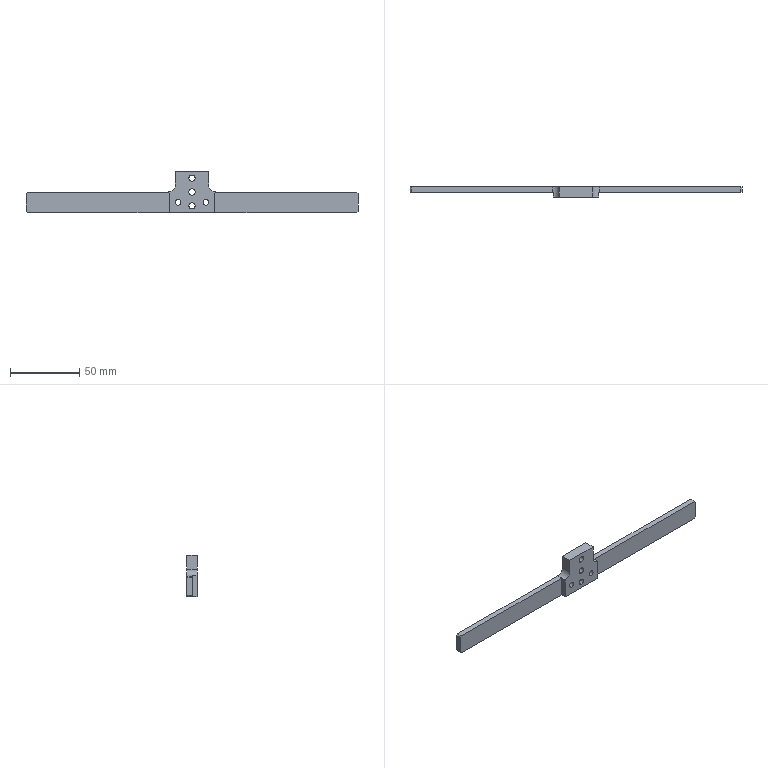Part | SolidWorks | features ICE 6, LPattern 2, Chamfer 1, Extrusion 1, Fillet 1, HoleWzd 1 | 1 solid | 30 faces | box 240 x 7.5 x 30 mm | volume 18359 mm3 | plane 18 | cylinder 12 | commonest cylinder face diameters 4.5 x6 4 x4 10 x2
STEP:
#1=CARTESIAN_POINT('',(-80.,-5.5,-9.5));
#2=VERTEX_POINT('',#1);
#3=CARTESIAN_POINT('',(-80.,-5.5,-5.5));
#4=VERTEX_POINT('',#3);
#5=CARTESIAN_POINT('',(-80.,-5.5,-7.5));
#6=DIRECTION('',(0.,1.,0.));
#7=DIRECTION('',(0.,0.,1.));
#8=AXIS2_PLACEMENT_3D('',#5,#6,#7);
#9=CIRCLE('',#8,2.);
#10=EDGE_CURVE('',#2,#4,#9,.T.);
#11=ORIENTED_EDGE('',*,*,#10,.F.);
#12=CARTESIAN_POINT('',(-80.,2.,-9.5));
#13=VERTEX_POINT('',#12);
#14=CARTESIAN_POINT('',(-80.,2.,-9.5));
#15=DIRECTION('',(0.,1.,0.));
#16=VECTOR('',#15,1000.);
#17=LINE('',#14,#16);
#18=EDGE_CURVE('',#2,#13,#17,.T.);
#19=ORIENTED_EDGE('',*,*,#18,.T.);
#20=CARTESIAN_POINT('',(-80.,2.,-5.5));
#21=VERTEX_POINT('',#20);
#22=CARTESIAN_POINT('',(-80.,2.,-7.5));
#23=DIRECTION('',(0.,1.,0.));
#24=DIRECTION('',(0.,0.,1.));
#25=AXIS2_PLACEMENT_3D('',#22,#23,#24);
#26=CIRCLE('',#25,2.);
#27=EDGE_CURVE('',#13,#21,#26,.T.);
#28=ORIENTED_EDGE('',*,*,#27,.T.);
#29=CARTESIAN_POINT('',(-80.,2.,-5.5));
#30=DIRECTION('',(0.,1.,0.));
#31=VECTOR('',#30,1000.);
#32=LINE('',#29,#31);
#33=EDGE_CURVE('',#4,#21,#32,.T.);
#34=ORIENTED_EDGE('',*,*,#33,.F.);
#35=EDGE_LOOP('',(#11,#19,#28,#34));
#36=FACE_OUTER_BOUND('',#35,.T.);
#37=CARTESIAN_POINT('',(-80.,2.,-7.5));
#38=DIRECTION('',(0.,1.,0.));
#39=DIRECTION('',(0.,0.,1.));
#40=AXIS2_PLACEMENT_3D('',#37,#38,#39);
#41=CYLINDRICAL_SURFACE('',#40,2.);
#42=ADVANCED_FACE('',(#36),#41,.F.);
#43=CARTESIAN_POINT('',(-60.,-5.5,-9.5));
#44=VERTEX_POINT('',#43);
#45=CARTESIAN_POINT('',(-60.,-5.5,-5.5));
#46=VERTEX_POINT('',#45);
#47=CARTESIAN_POINT('',(-60.,-5.5,-7.5));
#48=DIRECTION('',(0.,1.,0.));
#49=DIRECTION('',(0.,0.,1.));
#50=AXIS2_PLACEMENT_3D('',#47,#48,#49);
#51=CIRCLE('',#50,2.);
#52=EDGE_CURVE('',#44,#46,#51,.T.);
#53=ORIENTED_EDGE('',*,*,#52,.F.);
#54=CARTESIAN_POINT('',(-60.,2.,-9.5));
#55=VERTEX_POINT('',#54);
#56=CARTESIAN_POINT('',(-60.,2.,-9.5));
#57=DIRECTION('',(0.,1.,0.));
#58=VECTOR('',#57,1000.);
#59=LINE('',#56,#58);
#60=EDGE_CURVE('',#44,#55,#59,.T.);
#61=ORIENTED_EDGE('',*,*,#60,.T.);
#62=CARTESIAN_POINT('',(-60.,2.,-5.5));
#63=VERTEX_POINT('',#62);
#64=CARTESIAN_POINT('',(-60.,2.,-7.5));
#65=DIRECTION('',(0.,1.,0.));
#66=DIRECTION('',(0.,0.,1.));
#67=AXIS2_PLACEMENT_3D('',#64,#65,#66);
#68=CIRCLE('',#67,2.);
#69=EDGE_CURVE('',#55,#63,#68,.T.);
#70=ORIENTED_EDGE('',*,*,#69,.T.);
#71=CARTESIAN_POINT('',(-60.,2.,-5.5));
#72=DIRECTION('',(0.,1.,0.));
#73=VECTOR('',#72,1000.);
#74=LINE('',#71,#73);
#75=EDGE_CURVE('',#46,#63,#74,.T.);
#76=ORIENTED_EDGE('',*,*,#75,.F.);
#77=EDGE_LOOP('',(#53,#61,#70,#76));
#78=FACE_OUTER_BOUND('',#77,.T.);
#79=CARTESIAN_POINT('',(-60.,2.,-7.5));
#80=DIRECTION('',(0.,1.,0.));
#81=DIRECTION('',(0.,0.,1.));
#82=AXIS2_PLACEMENT_3D('',#79,#80,#81);
#83=CYLINDRICAL_SURFACE('',#82,2.);
#84=ADVANCED_FACE('',(#78),#83,.F.);
#85=CARTESIAN_POINT('',(-70.,-5.5,-7.75));
#86=VERTEX_POINT('',#85);
#87=CARTESIAN_POINT('',(-70.,-5.5,-12.25));
#88=VERTEX_POINT('',#87);
#89=CARTESIAN_POINT('',(-70.,-5.5,-10.));
#90=DIRECTION('',(0.,-1.,0.));
#91=DIRECTION('',(0.,0.,-1.));
#92=AXIS2_PLACEMENT_3D('',#89,#90,#91);
#93=CIRCLE('',#92,2.25);
#94=EDGE_CURVE('',#86,#88,#93,.T.);
#95=ORIENTED_EDGE('',*,*,#94,.T.);
#96=CARTESIAN_POINT('',(-70.,2.,-12.25));
#97=VERTEX_POINT('',#96);
#98=CARTESIAN_POINT('',(-70.,-5.5,-12.25));
#99=DIRECTION('',(0.,1.,0.));
#100=VECTOR('',#99,1000.);
#101=LINE('',#98,#100);
#102=EDGE_CURVE('',#88,#97,#101,.T.);
#103=ORIENTED_EDGE('',*,*,#102,.T.);
#104=CARTESIAN_POINT('',(-70.,2.,-7.75));
#105=VERTEX_POINT('',#104);
#106=CARTESIAN_POINT('',(-70.,2.,-10.));
#107=DIRECTION('',(0.,1.,0.));
#108=DIRECTION('',(0.,0.,1.));
#109=AXIS2_PLACEMENT_3D('',#106,#107,#108);
#110=CIRCLE('',#109,2.25);
#111=EDGE_CURVE('',#97,#105,#110,.T.);
#112=ORIENTED_EDGE('',*,*,#111,.T.);
#113=CARTESIAN_POINT('',(-70.,-5.5,-7.75));
#114=DIRECTION('',(0.,1.,0.));
#115=VECTOR('',#114,1000.);
#116=LINE('',#113,#115);
#117=EDGE_CURVE('',#86,#105,#116,.T.);
#118=ORIENTED_EDGE('',*,*,#117,.F.);
#119=EDGE_LOOP('',(#95,#103,#112,#118));
#120=FACE_OUTER_BOUND('',#119,.T.);
#121=CARTESIAN_POINT('',(-70.,-5.5,-10.));
#122=DIRECTION('',(0.,1.,0.));
#123=DIRECTION('',(0.,0.,1.));
#124=AXIS2_PLACEMENT_3D('',#121,#122,#123);
#125=CYLINDRICAL_SURFACE('',#124,2.25);
#126=ADVANCED_FACE('',(#120),#125,.F.);
#127=CARTESIAN_POINT('',(-70.,-5.5,2.25));
#128=VERTEX_POINT('',#127);
#129=CARTESIAN_POINT('',(-70.,-5.5,-2.25));
#130=VERTEX_POINT('',#129);
#131=CARTESIAN_POINT('',(-70.,-5.5,0.));
#132=DIRECTION('',(0.,-1.,0.));
#133=DIRECTION('',(0.,0.,-1.));
#134=AXIS2_PLACEMENT_3D('',#131,#132,#133);
#135=CIRCLE('',#134,2.25);
#136=EDGE_CURVE('',#128,#130,#135,.T.);
#137=ORIENTED_EDGE('',*,*,#136,.T.);
#138=CARTESIAN_POINT('',(-70.,2.,-2.25));
#139=VERTEX_POINT('',#138);
#140=CARTESIAN_POINT('',(-70.,-5.5,-2.25));
#141=DIRECTION('',(0.,1.,0.));
#142=VECTOR('',#141,1000.);
#143=LINE('',#140,#142);
#144=EDGE_CURVE('',#130,#139,#143,.T.);
#145=ORIENTED_EDGE('',*,*,#144,.T.);
#146=CARTESIAN_POINT('',(-70.,2.,2.25));
#147=VERTEX_POINT('',#146);
#148=CARTESIAN_POINT('',(-70.,2.,0.));
#149=DIRECTION('',(0.,1.,0.));
#150=DIRECTION('',(0.,0.,1.));
#151=AXIS2_PLACEMENT_3D('',#148,#149,#150);
#152=CIRCLE('',#151,2.25);
#153=EDGE_CURVE('',#139,#147,#152,.T.);
#154=ORIENTED_EDGE('',*,*,#153,.T.);
#155=CARTESIAN_POINT('',(-70.,-5.5,2.25));
#156=DIRECTION('',(0.,1.,0.));
#157=VECTOR('',#156,1000.);
#158=LINE('',#155,#157);
#159=EDGE_CURVE('',#128,#147,#158,.T.);
#160=ORIENTED_EDGE('',*,*,#159,.F.);
#161=EDGE_LOOP('',(#137,#145,#154,#160));
#162=FACE_OUTER_BOUND('',#161,.T.);
#163=CARTESIAN_POINT('',(-70.,-5.5,0.));
#164=DIRECTION('',(0.,1.,0.));
#165=DIRECTION('',(0.,0.,1.));
#166=AXIS2_PLACEMENT_3D('',#163,#164,#165);
#167=CYLINDRICAL_SURFACE('',#166,2.25);
#168=ADVANCED_FACE('',(#162),#167,.F.);
#169=CARTESIAN_POINT('',(-70.,-5.5,12.25));
#170=VERTEX_POINT('',#169);
#171=CARTESIAN_POINT('',(-70.,-5.5,7.75));
#172=VERTEX_POINT('',#171);
#173=CARTESIAN_POINT('',(-70.,-5.5,10.));
#174=DIRECTION('',(0.,-1.,0.));
#175=DIRECTION('',(0.,0.,-1.));
#176=AXIS2_PLACEMENT_3D('',#173,#174,#175);
#177=CIRCLE('',#176,2.25);
#178=EDGE_CURVE('',#170,#172,#177,.T.);
#179=ORIENTED_EDGE('',*,*,#178,.T.);
#180=CARTESIAN_POINT('',(-70.,2.,7.75));
#181=VERTEX_POINT('',#180);
#182=CARTESIAN_POINT('',(-70.,-5.5,7.75));
#183=DIRECTION('',(0.,1.,0.));
#184=VECTOR('',#183,1000.);
#185=LINE('',#182,#184);
#186=EDGE_CURVE('',#172,#181,#185,.T.);
#187=ORIENTED_EDGE('',*,*,#186,.T.);
#188=CARTESIAN_POINT('',(-70.,2.,12.25));
#189=VERTEX_POINT('',#188);
#190=CARTESIAN_POINT('',(-70.,2.,10.));
#191=DIRECTION('',(0.,1.,0.));
#192=DIRECTION('',(0.,0.,1.));
#193=AXIS2_PLACEMENT_3D('',#190,#191,#192);
#194=CIRCLE('',#193,2.25);
#195=EDGE_CURVE('',#181,#189,#194,.T.);
#196=ORIENTED_EDGE('',*,*,#195,.T.);
#197=CARTESIAN_POINT('',(-70.,-5.5,12.25));
#198=DIRECTION('',(0.,1.,0.));
#199=VECTOR('',#198,1000.);
#200=LINE('',#197,#199);
#201=EDGE_CURVE('',#170,#189,#200,.T.);
#202=ORIENTED_EDGE('',*,*,#201,.F.);
#203=EDGE_LOOP('',(#179,#187,#196,#202));
#204=FACE_OUTER_BOUND('',#203,.T.);
#205=CARTESIAN_POINT('',(-70.,-5.5,10.));
#206=DIRECTION('',(0.,1.,0.));
#207=DIRECTION('',(0.,0.,1.));
#208=AXIS2_PLACEMENT_3D('',#205,#206,#207);
#209=CYLINDRICAL_SURFACE('',#208,2.25);
#210=ADVANCED_FACE('',(#204),#209,.F.);
#211=CARTESIAN_POINT('',(-80.,-5.5,-7.5));
#212=DIRECTION('',(0.,1.,0.));
#213=DIRECTION('',(0.,0.,1.));
#214=AXIS2_PLACEMENT_3D('',#211,#212,#213);
#215=CIRCLE('',#214,2.);
#216=EDGE_CURVE('',#4,#2,#215,.T.);
#217=ORIENTED_EDGE('',*,*,#216,.T.);
#218=ORIENTED_EDGE('',*,*,#10,.T.);
#219=EDGE_LOOP('',(#217,#218));
#220=FACE_BOUND('',#219,.T.);
#221=ORIENTED_EDGE('',*,*,#94,.F.);
#222=CARTESIAN_POINT('',(-70.,-5.5,-10.));
#223=DIRECTION('',(0.,-1.,0.));
#224=DIRECTION('',(0.,0.,-1.));
#225=AXIS2_PLACEMENT_3D('',#222,#223,#224);
#226=CIRCLE('',#225,2.25);
#227=EDGE_CURVE('',#88,#86,#226,.T.);
#228=ORIENTED_EDGE('',*,*,#227,.F.);
#229=EDGE_LOOP('',(#221,#228));
#230=FACE_BOUND('',#229,.T.);
#231=ORIENTED_EDGE('',*,*,#178,.F.);
#232=CARTESIAN_POINT('',(-70.,-5.5,10.));
#233=DIRECTION('',(0.,-1.,0.));
#234=DIRECTION('',(0.,0.,-1.));
#235=AXIS2_PLACEMENT_3D('',#232,#233,#234);
#236=CIRCLE('',#235,2.25);
#237=EDGE_CURVE('',#172,#170,#236,.T.);
#238=ORIENTED_EDGE('',*,*,#237,.F.);
#239=EDGE_LOOP('',(#231,#238));
#240=FACE_BOUND('',#239,.T.);
#241=ORIENTED_EDGE('',*,*,#136,.F.);
#242=CARTESIAN_POINT('',(-70.,-5.5,0.));
#243=DIRECTION('',(0.,-1.,0.));
#244=DIRECTION('',(0.,0.,-1.));
#245=AXIS2_PLACEMENT_3D('',#242,#243,#244);
#246=CIRCLE('',#245,2.25);
#247=EDGE_CURVE('',#130,#128,#246,.T.);
#248=ORIENTED_EDGE('',*,*,#247,.F.);
#249=EDGE_LOOP('',(#241,#248));
#250=FACE_BOUND('',#249,.T.);
#251=CARTESIAN_POINT('',(-82.,-5.5,5.));
#252=VERTEX_POINT('',#251);
#253=CARTESIAN_POINT('',(-82.,-5.5,15.));
#254=VERTEX_POINT('',#253);
#255=CARTESIAN_POINT('',(-82.,-5.5,-15.));
#256=DIRECTION('',(0.,0.,1.));
#257=VECTOR('',#256,1000.);
#258=LINE('',#255,#257);
#259=EDGE_CURVE('',#252,#254,#258,.T.);
#260=ORIENTED_EDGE('',*,*,#259,.F.);
#261=CARTESIAN_POINT('',(-86.5,-5.5,0.02506));
#262=VERTEX_POINT('',#261);
#263=CARTESIAN_POINT('',(-87.,-5.5,5.));
#264=DIRECTION('',(0.,-1.,0.));
#265=DIRECTION('',(0.,0.,-1.));
#266=AXIS2_PLACEMENT_3D('',#263,#264,#265);
#267=CIRCLE('',#266,5.);
#268=EDGE_CURVE('',#262,#252,#267,.T.);
#269=ORIENTED_EDGE('',*,*,#268,.F.);
#270=CARTESIAN_POINT('',(-86.5,-5.5,-15.));
#271=VERTEX_POINT('',#270);
#272=CARTESIAN_POINT('',(-86.5,-5.5,-15.));
#273=DIRECTION('',(0.,0.,-1.));
#274=VECTOR('',#273,1000.);
#275=LINE('',#272,#274);
#276=EDGE_CURVE('',#262,#271,#275,.T.);
#277=ORIENTED_EDGE('',*,*,#276,.T.);
#278=CARTESIAN_POINT('',(-53.5,-5.5,-15.));
#279=VERTEX_POINT('',#278);
#280=CARTESIAN_POINT('',(-82.,-5.5,-15.));
#281=DIRECTION('',(1.,0.,0.));
#282=VECTOR('',#281,1000.);
#283=LINE('',#280,#282);
#284=EDGE_CURVE('',#271,#279,#283,.T.);
#285=ORIENTED_EDGE('',*,*,#284,.T.);
#286=CARTESIAN_POINT('',(-53.5,-5.5,0.02506));
#287=VERTEX_POINT('',#286);
#288=CARTESIAN_POINT('',(-53.5,-5.5,-15.));
#289=DIRECTION('',(0.,0.,1.));
#290=VECTOR('',#289,1000.);
#291=LINE('',#288,#290);
#292=EDGE_CURVE('',#279,#287,#291,.T.);
#293=ORIENTED_EDGE('',*,*,#292,.T.);
#294=CARTESIAN_POINT('',(-58.,-5.5,5.));
#295=VERTEX_POINT('',#294);
#296=CARTESIAN_POINT('',(-53.,-5.5,5.));
#297=DIRECTION('',(0.,-1.,0.));
#298=DIRECTION('',(0.,0.,-1.));
#299=AXIS2_PLACEMENT_3D('',#296,#297,#298);
#300=CIRCLE('',#299,5.);
#301=EDGE_CURVE('',#295,#287,#300,.T.);
#302=ORIENTED_EDGE('',*,*,#301,.F.);
#303=CARTESIAN_POINT('',(-58.,-5.5,15.));
#304=VERTEX_POINT('',#303);
#305=CARTESIAN_POINT('',(-58.,-5.5,-15.));
#306=DIRECTION('',(0.,0.,-1.));
#307=VECTOR('',#306,1000.);
#308=LINE('',#305,#307);
#309=EDGE_CURVE('',#304,#295,#308,.T.);
#310=ORIENTED_EDGE('',*,*,#309,.F.);
#311=CARTESIAN_POINT('',(-82.,-5.5,15.));
#312=DIRECTION('',(-1.,0.,0.));
#313=VECTOR('',#312,1000.);
#314=LINE('',#311,#313);
#315=EDGE_CURVE('',#304,#254,#314,.T.);
#316=ORIENTED_EDGE('',*,*,#315,.T.);
#317=EDGE_LOOP('',(#260,#269,#277,#285,#293,#302,#310,#316));
#318=FACE_OUTER_BOUND('',#317,.T.);
#319=CARTESIAN_POINT('',(-60.,-5.5,-7.5));
#320=DIRECTION('',(0.,1.,0.));
#321=DIRECTION('',(0.,0.,1.));
#322=AXIS2_PLACEMENT_3D('',#319,#320,#321);
#323=CIRCLE('',#322,2.);
#324=EDGE_CURVE('',#46,#44,#323,.T.);
#325=ORIENTED_EDGE('',*,*,#324,.T.);
#326=ORIENTED_EDGE('',*,*,#52,.T.);
#327=EDGE_LOOP('',(#325,#326));
#328=FACE_BOUND('',#327,.T.);
#329=CARTESIAN_POINT('',(-82.,-5.5,-15.));
#330=DIRECTION('',(0.,-1.,0.));
#331=DIRECTION('',(0.,0.,-1.));
#332=AXIS2_PLACEMENT_3D('',#329,#330,#331);
#333=PLANE('',#332);
#334=ADVANCED_FACE('',(#220,#230,#240,#250,#318,#328),#333,.T.);
#335=CARTESIAN_POINT('',(-189.,-2.,-15.));
#336=VERTEX_POINT('',#335);
#337=CARTESIAN_POINT('',(-86.5,-2.,-15.));
#338=VERTEX_POINT('',#337);
#339=CARTESIAN_POINT('',(-69.,-2.,-15.));
#340=DIRECTION('',(1.,0.,0.));
#341=VECTOR('',#340,1000.);
#342=LINE('',#339,#341);
#343=EDGE_CURVE('',#336,#338,#342,.T.);
#344=ORIENTED_EDGE('',*,*,#343,.T.);
#345=CARTESIAN_POINT('',(-86.5,-2.,0.02506));
#346=VERTEX_POINT('',#345);
#347=CARTESIAN_POINT('',(-86.5,-2.,-15.));
#348=DIRECTION('',(0.,0.,-1.));
#349=VECTOR('',#348,1000.);
#350=LINE('',#347,#349);
#351=EDGE_CURVE('',#346,#338,#350,.T.);
#352=ORIENTED_EDGE('',*,*,#351,.F.);
#353=CARTESIAN_POINT('',(-87.,-2.,0.));
#354=VERTEX_POINT('',#353);
#355=CARTESIAN_POINT('',(-87.,-2.,5.));
#356=DIRECTION('',(0.,1.,0.));
#357=DIRECTION('',(0.,0.,1.));
#358=AXIS2_PLACEMENT_3D('',#355,#356,#357);
#359=CIRCLE('',#358,5.);
#360=EDGE_CURVE('',#346,#354,#359,.T.);
#361=ORIENTED_EDGE('',*,*,#360,.T.);
#362=CARTESIAN_POINT('',(-189.,-2.,0.));
#363=VERTEX_POINT('',#362);
#364=CARTESIAN_POINT('',(-190.,-2.,0.));
#365=DIRECTION('',(1.,0.,0.));
#366=VECTOR('',#365,1000.);
#367=LINE('',#364,#366);
#368=EDGE_CURVE('',#363,#354,#367,.T.);
#369=ORIENTED_EDGE('',*,*,#368,.F.);
#370=CARTESIAN_POINT('',(-190.,-2.,-1.));
#371=VERTEX_POINT('',#370);
#372=CARTESIAN_POINT('',(-190.,-2.,-1.));
#373=DIRECTION('',(-0.7071,0.,-0.7071));
#374=VECTOR('',#373,1000.);
#375=LINE('',#372,#374);
#376=EDGE_CURVE('',#363,#371,#375,.T.);
#377=ORIENTED_EDGE('',*,*,#376,.T.);
#378=CARTESIAN_POINT('',(-190.,-2.,-14.));
#379=VERTEX_POINT('',#378);
#380=CARTESIAN_POINT('',(-190.,-2.,-15.));
#381=DIRECTION('',(0.,0.,1.));
#382=VECTOR('',#381,1000.);
#383=LINE('',#380,#382);
#384=EDGE_CURVE('',#379,#371,#383,.T.);
#385=ORIENTED_EDGE('',*,*,#384,.F.);
#386=CARTESIAN_POINT('',(-189.,-2.,-15.));
#387=DIRECTION('',(0.7071,0.,-0.7071));
#388=VECTOR('',#387,1000.);
#389=LINE('',#386,#388);
#390=EDGE_CURVE('',#379,#336,#389,.T.);
#391=ORIENTED_EDGE('',*,*,#390,.T.);
#392=EDGE_LOOP('',(#344,#352,#361,#369,#377,#385,#391));
#393=FACE_OUTER_BOUND('',#392,.T.);
#394=CARTESIAN_POINT('',(-53.,-2.,5.));
#395=DIRECTION('',(0.,1.,0.));
#396=DIRECTION('',(0.,0.,1.));
#397=AXIS2_PLACEMENT_3D('',#394,#395,#396);
#398=PLANE('',#397);
#399=ADVANCED_FACE('',(#393),#398,.F.);
#400=CARTESIAN_POINT('',(-53.,-2.,0.));
#401=VERTEX_POINT('',#400);
#402=CARTESIAN_POINT('',(-53.5,-2.,0.02506));
#403=VERTEX_POINT('',#402);
#404=CARTESIAN_POINT('',(-53.,-2.,5.));
#405=DIRECTION('',(0.,1.,0.));
#406=DIRECTION('',(0.,0.,1.));
#407=AXIS2_PLACEMENT_3D('',#404,#405,#406);
#408=CIRCLE('',#407,5.);
#409=EDGE_CURVE('',#401,#403,#408,.T.);
#410=ORIENTED_EDGE('',*,*,#409,.T.);
#411=CARTESIAN_POINT('',(-53.5,-2.,-15.));
#412=VERTEX_POINT('',#411);
#413=CARTESIAN_POINT('',(-53.5,-2.,-15.));
#414=DIRECTION('',(0.,0.,1.));
#415=VECTOR('',#414,1000.);
#416=LINE('',#413,#415);
#417=EDGE_CURVE('',#412,#403,#416,.T.);
#418=ORIENTED_EDGE('',*,*,#417,.F.);
#419=CARTESIAN_POINT('',(49.,-2.,-15.));
#420=VERTEX_POINT('',#419);
#421=CARTESIAN_POINT('',(-69.,-2.,-15.));
#422=DIRECTION('',(1.,0.,0.));
#423=VECTOR('',#422,1000.);
#424=LINE('',#421,#423);
#425=EDGE_CURVE('',#412,#420,#424,.T.);
#426=ORIENTED_EDGE('',*,*,#425,.T.);
#427=CARTESIAN_POINT('',(50.,-2.,-14.));
#428=VERTEX_POINT('',#427);
#429=CARTESIAN_POINT('',(50.,-2.,-14.));
#430=DIRECTION('',(0.7071,0.,0.7071));
#431=VECTOR('',#430,1000.);
#432=LINE('',#429,#431);
#433=EDGE_CURVE('',#420,#428,#432,.T.);
#434=ORIENTED_EDGE('',*,*,#433,.T.);
#435=CARTESIAN_POINT('',(50.,-2.,-1.));
#436=VERTEX_POINT('',#435);
#437=CARTESIAN_POINT('',(50.,-2.,5.));
#438=DIRECTION('',(0.,0.,1.));
#439=VECTOR('',#438,1000.);
#440=LINE('',#437,#439);
#441=EDGE_CURVE('',#428,#436,#440,.T.);
#442=ORIENTED_EDGE('',*,*,#441,.T.);
#443=CARTESIAN_POINT('',(49.,-2.,0.));
#444=VERTEX_POINT('',#443);
#445=CARTESIAN_POINT('',(50.,-2.,-1.));
#446=DIRECTION('',(-0.7071,0.,0.7071));
#447=VECTOR('',#446,1000.);
#448=LINE('',#445,#447);
#449=EDGE_CURVE('',#436,#444,#448,.T.);
#450=ORIENTED_EDGE('',*,*,#449,.T.);
#451=CARTESIAN_POINT('',(69.,-2.,0.));
#452=DIRECTION('',(-1.,0.,0.));
#453=VECTOR('',#452,1000.);
#454=LINE('',#451,#453);
#455=EDGE_CURVE('',#444,#401,#454,.T.);
#456=ORIENTED_EDGE('',*,*,#455,.T.);
#457=EDGE_LOOP('',(#410,#418,#426,#434,#442,#450,#456));
#458=FACE_OUTER_BOUND('',#457,.T.);
#459=CARTESIAN_POINT('',(-53.,-2.,5.));
#460=DIRECTION('',(0.,1.,0.));
#461=DIRECTION('',(0.,0.,1.));
#462=AXIS2_PLACEMENT_3D('',#459,#460,#461);
#463=PLANE('',#462);
#464=ADVANCED_FACE('',(#458),#463,.F.);
#465=CARTESIAN_POINT('',(-58.,2.,15.));
#466=VERTEX_POINT('',#465);
#467=CARTESIAN_POINT('',(-58.,2.,15.));
#468=DIRECTION('',(0.,-1.,0.));
#469=VECTOR('',#468,1000.);
#470=LINE('',#467,#469);
#471=EDGE_CURVE('',#466,#304,#470,.T.);
#472=ORIENTED_EDGE('',*,*,#471,.T.);
#473=ORIENTED_EDGE('',*,*,#309,.T.);
#474=CARTESIAN_POINT('',(-58.,2.,5.));
#475=VERTEX_POINT('',#474);
#476=CARTESIAN_POINT('',(-58.,2.,5.));
#477=DIRECTION('',(0.,-1.,0.));
#478=VECTOR('',#477,1000.);
#479=LINE('',#476,#478);
#480=EDGE_CURVE('',#475,#295,#479,.T.);
#481=ORIENTED_EDGE('',*,*,#480,.F.);
#482=CARTESIAN_POINT('',(-58.,2.,5.));
#483=DIRECTION('',(0.,0.,1.));
#484=VECTOR('',#483,1000.);
#485=LINE('',#482,#484);
#486=EDGE_CURVE('',#475,#466,#485,.T.);
#487=ORIENTED_EDGE('',*,*,#486,.T.);
#488=EDGE_LOOP('',(#472,#473,#481,#487));
#489=FACE_OUTER_BOUND('',#488,.T.);
#490=CARTESIAN_POINT('',(-58.,2.,5.));
#491=DIRECTION('',(1.,0.,0.));
#492=DIRECTION('',(0.,0.,-1.));
#493=AXIS2_PLACEMENT_3D('',#490,#491,#492);
#494=PLANE('',#493);
#495=ADVANCED_FACE('',(#489),#494,.T.);
#496=ORIENTED_EDGE('',*,*,#409,.F.);
#497=CARTESIAN_POINT('',(-53.,2.,0.));
#498=VERTEX_POINT('',#497);
#499=CARTESIAN_POINT('',(-53.,2.,0.));
#500=DIRECTION('',(0.,-1.,0.));
#501=VECTOR('',#500,1000.);
#502=LINE('',#499,#501);
#503=EDGE_CURVE('',#498,#401,#502,.T.);
#504=ORIENTED_EDGE('',*,*,#503,.F.);
#505=CARTESIAN_POINT('',(-53.,2.,5.));
#506=DIRECTION('',(0.,1.,0.));
#507=DIRECTION('',(0.,0.,1.));
#508=AXIS2_PLACEMENT_3D('',#505,#506,#507);
#509=CIRCLE('',#508,5.);
#510=EDGE_CURVE('',#498,#475,#509,.T.);
#511=ORIENTED_EDGE('',*,*,#510,.T.);
#512=ORIENTED_EDGE('',*,*,#480,.T.);
#513=ORIENTED_EDGE('',*,*,#301,.T.);
#514=CARTESIAN_POINT('',(-53.5,-12.,0.02506));
#515=DIRECTION('',(0.,1.,0.));
#516=VECTOR('',#515,1000.);
#517=LINE('',#514,#516);
#518=EDGE_CURVE('',#287,#403,#517,.T.);
#519=ORIENTED_EDGE('',*,*,#518,.T.);
#520=EDGE_LOOP('',(#496,#504,#511,#512,#513,#519));
#521=FACE_OUTER_BOUND('',#520,.T.);
#522=CARTESIAN_POINT('',(-53.,2.,5.));
#523=DIRECTION('',(0.,-1.,0.));
#524=DIRECTION('',(0.,0.,-1.));
#525=AXIS2_PLACEMENT_3D('',#522,#523,#524);
#526=CYLINDRICAL_SURFACE('',#525,5.);
#527=ADVANCED_FACE('',(#521),#526,.F.);
#528=ORIENTED_EDGE('',*,*,#455,.F.);
#529=CARTESIAN_POINT('',(49.,2.,0.));
#530=VERTEX_POINT('',#529);
#531=CARTESIAN_POINT('',(49.,2.,0.));
#532=DIRECTION('',(0.,1.,0.));
#533=VECTOR('',#532,1000.);
#534=LINE('',#531,#533);
#535=EDGE_CURVE('',#444,#530,#534,.T.);
#536=ORIENTED_EDGE('',*,*,#535,.T.);
#537=CARTESIAN_POINT('',(69.,2.,0.));
#538=DIRECTION('',(-1.,0.,0.));
#539=VECTOR('',#538,1000.);
#540=LINE('',#537,#539);
#541=EDGE_CURVE('',#530,#498,#540,.T.);
#542=ORIENTED_EDGE('',*,*,#541,.T.);
#543=ORIENTED_EDGE('',*,*,#503,.T.);
#544=EDGE_LOOP('',(#528,#536,#542,#543));
#545=FACE_OUTER_BOUND('',#544,.T.);
#546=CARTESIAN_POINT('',(69.,2.,0.));
#547=DIRECTION('',(0.,0.,1.));
#548=DIRECTION('',(1.,0.,0.));
#549=AXIS2_PLACEMENT_3D('',#546,#547,#548);
#550=PLANE('',#549);
#551=ADVANCED_FACE('',(#545),#550,.T.);
#552=ORIENTED_EDGE('',*,*,#425,.F.);
#553=CARTESIAN_POINT('',(-53.5,28.336,-15.));
#554=DIRECTION('',(0.,-1.,0.));
#555=VECTOR('',#554,1000.);
#556=LINE('',#553,#555);
#557=EDGE_CURVE('',#412,#279,#556,.T.);
#558=ORIENTED_EDGE('',*,*,#557,.T.);
#559=ORIENTED_EDGE('',*,*,#284,.F.);
#560=CARTESIAN_POINT('',(-86.5,28.336,-15.));
#561=DIRECTION('',(0.,-1.,0.));
#562=VECTOR('',#561,1000.);
#563=LINE('',#560,#562);
#564=EDGE_CURVE('',#338,#271,#563,.T.);
#565=ORIENTED_EDGE('',*,*,#564,.F.);
#566=ORIENTED_EDGE('',*,*,#343,.F.);
#567=CARTESIAN_POINT('',(-189.,2.,-15.));
#568=VERTEX_POINT('',#567);
#569=CARTESIAN_POINT('',(-189.,2.,-15.));
#570=DIRECTION('',(0.,1.,0.));
#571=VECTOR('',#570,1000.);
#572=LINE('',#569,#571);
#573=EDGE_CURVE('',#336,#568,#572,.T.);
#574=ORIENTED_EDGE('',*,*,#573,.T.);
#575=CARTESIAN_POINT('',(49.,2.,-15.));
#576=VERTEX_POINT('',#575);
#577=CARTESIAN_POINT('',(-69.,2.,-15.));
#578=DIRECTION('',(1.,0.,0.));
#579=VECTOR('',#578,1000.);
#580=LINE('',#577,#579);
#581=EDGE_CURVE('',#568,#576,#580,.T.);
#582=ORIENTED_EDGE('',*,*,#581,.T.);
#583=CARTESIAN_POINT('',(49.,-2.,-15.));
#584=DIRECTION('',(0.,-1.,0.));
#585=VECTOR('',#584,1000.);
#586=LINE('',#583,#585);
#587=EDGE_CURVE('',#576,#420,#586,.T.);
#588=ORIENTED_EDGE('',*,*,#587,.T.);
#589=EDGE_LOOP('',(#552,#558,#559,#565,#566,#574,#582,#588));
#590=FACE_OUTER_BOUND('',#589,.T.);
#591=CARTESIAN_POINT('',(-69.,2.,-15.));
#592=DIRECTION('',(0.,0.,-1.));
#593=DIRECTION('',(-1.,0.,0.));
#594=AXIS2_PLACEMENT_3D('',#591,#592,#593);
#595=PLANE('',#594);
#596=ADVANCED_FACE('',(#590),#595,.T.);
#597=CARTESIAN_POINT('',(-82.,2.,15.));
#598=VERTEX_POINT('',#597);
#599=CARTESIAN_POINT('',(-82.,-2.,15.));
#600=DIRECTION('',(0.,1.,0.));
#601=VECTOR('',#600,1000.);
#602=LINE('',#599,#601);
#603=EDGE_CURVE('',#254,#598,#602,.T.);
#604=ORIENTED_EDGE('',*,*,#603,.F.);
#605=ORIENTED_EDGE('',*,*,#315,.F.);
#606=ORIENTED_EDGE('',*,*,#471,.F.);
#607=CARTESIAN_POINT('',(-59.,2.,15.));
#608=DIRECTION('',(-1.,0.,0.));
#609=VECTOR('',#608,1000.);
#610=LINE('',#607,#609);
#611=EDGE_CURVE('',#466,#598,#610,.T.);
#612=ORIENTED_EDGE('',*,*,#611,.T.);
#613=EDGE_LOOP('',(#604,#605,#606,#612));
#614=FACE_OUTER_BOUND('',#613,.T.);
#615=CARTESIAN_POINT('',(-69.,2.,15.));
#616=DIRECTION('',(0.,0.,1.));
#617=DIRECTION('',(1.,0.,0.));
#618=AXIS2_PLACEMENT_3D('',#615,#616,#617);
#619=PLANE('',#618);
#620=ADVANCED_FACE('',(#614),#619,.T.);
#621=CARTESIAN_POINT('',(-80.,2.,-7.5));
#622=DIRECTION('',(0.,1.,0.));
#623=DIRECTION('',(0.,0.,1.));
#624=AXIS2_PLACEMENT_3D('',#621,#622,#623);
#625=CIRCLE('',#624,2.);
#626=EDGE_CURVE('',#21,#13,#625,.T.);
#627=ORIENTED_EDGE('',*,*,#626,.F.);
#628=ORIENTED_EDGE('',*,*,#27,.F.);
#629=EDGE_LOOP('',(#627,#628));
#630=FACE_BOUND('',#629,.T.);
#631=CARTESIAN_POINT('',(-60.,2.,-7.5));
#632=DIRECTION('',(0.,1.,0.));
#633=DIRECTION('',(0.,0.,1.));
#634=AXIS2_PLACEMENT_3D('',#631,#632,#633);
#635=CIRCLE('',#634,2.);
#636=EDGE_CURVE('',#63,#55,#635,.T.);
#637=ORIENTED_EDGE('',*,*,#636,.F.);
#638=ORIENTED_EDGE('',*,*,#69,.F.);
#639=EDGE_LOOP('',(#637,#638));
#640=FACE_BOUND('',#639,.T.);
#641=CARTESIAN_POINT('',(50.,2.,-14.));
#642=VERTEX_POINT('',#641);
#643=CARTESIAN_POINT('',(50.,2.,-1.));
#644=VERTEX_POINT('',#643);
#645=CARTESIAN_POINT('',(50.,2.,5.));
#646=DIRECTION('',(0.,0.,1.));
#647=VECTOR('',#646,1000.);
#648=LINE('',#645,#647);
#649=EDGE_CURVE('',#642,#644,#648,.T.);
#650=ORIENTED_EDGE('',*,*,#649,.F.);
#651=CARTESIAN_POINT('',(8.,2.,-56.));
#652=DIRECTION('',(-0.7071,0.,-0.7071));
#653=VECTOR('',#652,1000.);
#654=LINE('',#651,#653);
#655=EDGE_CURVE('',#642,#576,#654,.T.);
#656=ORIENTED_EDGE('',*,*,#655,.T.);
#657=ORIENTED_EDGE('',*,*,#581,.F.);
#658=CARTESIAN_POINT('',(-190.,2.,-14.));
#659=VERTEX_POINT('',#658);
#660=CARTESIAN_POINT('',(-131.,2.,-73.));
#661=DIRECTION('',(-0.7071,0.,0.7071));
#662=VECTOR('',#661,1000.);
#663=LINE('',#660,#662);
#664=EDGE_CURVE('',#568,#659,#663,.T.);
#665=ORIENTED_EDGE('',*,*,#664,.T.);
#666=CARTESIAN_POINT('',(-190.,2.,-1.));
#667=VERTEX_POINT('',#666);
#668=CARTESIAN_POINT('',(-190.,2.,-15.));
#669=DIRECTION('',(0.,0.,1.));
#670=VECTOR('',#669,1000.);
#671=LINE('',#668,#670);
#672=EDGE_CURVE('',#659,#667,#671,.T.);
#673=ORIENTED_EDGE('',*,*,#672,.T.);
#674=CARTESIAN_POINT('',(-189.,2.,0.));
#675=VERTEX_POINT('',#674);
#676=CARTESIAN_POINT('',(-118.5,2.,70.5));
#677=DIRECTION('',(0.7071,0.,0.7071));
#678=VECTOR('',#677,1000.);
#679=LINE('',#676,#678);
#680=EDGE_CURVE('',#667,#675,#679,.T.);
#681=ORIENTED_EDGE('',*,*,#680,.T.);
#682=CARTESIAN_POINT('',(-87.,2.,0.));
#683=VERTEX_POINT('',#682);
#684=CARTESIAN_POINT('',(-190.,2.,0.));
#685=DIRECTION('',(1.,0.,0.));
#686=VECTOR('',#685,1000.);
#687=LINE('',#684,#686);
#688=EDGE_CURVE('',#675,#683,#687,.T.);
#689=ORIENTED_EDGE('',*,*,#688,.T.);
#690=CARTESIAN_POINT('',(-82.,2.,5.));
#691=VERTEX_POINT('',#690);
#692=CARTESIAN_POINT('',(-87.,2.,5.));
#693=DIRECTION('',(0.,-1.,0.));
#694=DIRECTION('',(0.,0.,1.));
#695=AXIS2_PLACEMENT_3D('',#692,#693,#694);
#696=CIRCLE('',#695,5.);
#697=EDGE_CURVE('',#683,#691,#696,.T.);
#698=ORIENTED_EDGE('',*,*,#697,.T.);
#699=CARTESIAN_POINT('',(-82.,2.,15.));
#700=DIRECTION('',(0.,0.,1.));
#701=VECTOR('',#700,1000.);
#702=LINE('',#699,#701);
#703=EDGE_CURVE('',#691,#598,#702,.T.);
#704=ORIENTED_EDGE('',*,*,#703,.T.);
#705=ORIENTED_EDGE('',*,*,#611,.F.);
#706=ORIENTED_EDGE('',*,*,#486,.F.);
#707=ORIENTED_EDGE('',*,*,#510,.F.);
#708=ORIENTED_EDGE('',*,*,#541,.F.);
#709=CARTESIAN_POINT('',(-4.5,2.,53.5));
#710=DIRECTION('',(0.7071,0.,-0.7071));
#711=VECTOR('',#710,1000.);
#712=LINE('',#709,#711);
#713=EDGE_CURVE('',#530,#644,#712,.T.);
#714=ORIENTED_EDGE('',*,*,#713,.T.);
#715=EDGE_LOOP('',(#650,#656,#657,#665,#673,#681,#689,#698,#704,#705,#706,#707,#708,#714));
#716=FACE_OUTER_BOUND('',#715,.T.);
#717=CARTESIAN_POINT('',(-70.,2.,0.));
#718=DIRECTION('',(0.,1.,0.));
#719=DIRECTION('',(0.,0.,1.));
#720=AXIS2_PLACEMENT_3D('',#717,#718,#719);
#721=CIRCLE('',#720,2.25);
#722=EDGE_CURVE('',#147,#139,#721,.T.);
#723=ORIENTED_EDGE('',*,*,#722,.F.);
#724=ORIENTED_EDGE('',*,*,#153,.F.);
#725=EDGE_LOOP('',(#723,#724));
#726=FACE_BOUND('',#725,.T.);
#727=CARTESIAN_POINT('',(-70.,2.,10.));
#728=DIRECTION('',(0.,1.,0.));
#729=DIRECTION('',(0.,0.,1.));
#730=AXIS2_PLACEMENT_3D('',#727,#728,#729);
#731=CIRCLE('',#730,2.25);
#732=EDGE_CURVE('',#189,#181,#731,.T.);
#733=ORIENTED_EDGE('',*,*,#732,.F.);
#734=ORIENTED_EDGE('',*,*,#195,.F.);
#735=EDGE_LOOP('',(#733,#734));
#736=FACE_BOUND('',#735,.T.);
#737=CARTESIAN_POINT('',(-70.,2.,-10.));
#738=DIRECTION('',(0.,1.,0.));
#739=DIRECTION('',(0.,0.,1.));
#740=AXIS2_PLACEMENT_3D('',#737,#738,#739);
#741=CIRCLE('',#740,2.25);
#742=EDGE_CURVE('',#105,#97,#741,.T.);
#743=ORIENTED_EDGE('',*,*,#742,.F.);
#744=ORIENTED_EDGE('',*,*,#111,.F.);
#745=EDGE_LOOP('',(#743,#744));
#746=FACE_BOUND('',#745,.T.);
#747=CARTESIAN_POINT('',(-53.,2.,5.));
#748=DIRECTION('',(0.,1.,0.));
#749=DIRECTION('',(0.,0.,1.));
#750=AXIS2_PLACEMENT_3D('',#747,#748,#749);
#751=PLANE('',#750);
#752=ADVANCED_FACE('',(#630,#640,#716,#726,#736,#746),#751,.T.);
#753=CARTESIAN_POINT('',(-82.,-2.,5.));
#754=DIRECTION('',(0.,-1.,0.));
#755=VECTOR('',#754,1000.);
#756=LINE('',#753,#755);
#757=EDGE_CURVE('',#691,#252,#756,.T.);
#758=ORIENTED_EDGE('',*,*,#757,.T.);
#759=ORIENTED_EDGE('',*,*,#259,.T.);
#760=ORIENTED_EDGE('',*,*,#603,.T.);
#761=ORIENTED_EDGE('',*,*,#703,.F.);
#762=EDGE_LOOP('',(#758,#759,#760,#761));
#763=FACE_OUTER_BOUND('',#762,.T.);
#764=CARTESIAN_POINT('',(-82.,-2.,15.));
#765=DIRECTION('',(-1.,0.,0.));
#766=DIRECTION('',(0.,0.,1.));
#767=AXIS2_PLACEMENT_3D('',#764,#765,#766);
#768=PLANE('',#767);
#769=ADVANCED_FACE('',(#763),#768,.T.);
#770=ORIENTED_EDGE('',*,*,#688,.F.);
#771=CARTESIAN_POINT('',(-189.,-2.,0.));
#772=DIRECTION('',(0.,-1.,0.));
#773=VECTOR('',#772,1000.);
#774=LINE('',#771,#773);
#775=EDGE_CURVE('',#675,#363,#774,.T.);
#776=ORIENTED_EDGE('',*,*,#775,.T.);
#777=ORIENTED_EDGE('',*,*,#368,.T.);
#778=CARTESIAN_POINT('',(-87.,2.,0.));
#779=DIRECTION('',(0.,1.,0.));
#780=VECTOR('',#779,1000.);
#781=LINE('',#778,#780);
#782=EDGE_CURVE('',#354,#683,#781,.T.);
#783=ORIENTED_EDGE('',*,*,#782,.T.);
#784=EDGE_LOOP('',(#770,#776,#777,#783));
#785=FACE_OUTER_BOUND('',#784,.T.);
#786=CARTESIAN_POINT('',(-190.,-2.,0.));
#787=DIRECTION('',(0.,0.,1.));
#788=DIRECTION('',(1.,0.,0.));
#789=AXIS2_PLACEMENT_3D('',#786,#787,#788);
#790=PLANE('',#789);
#791=ADVANCED_FACE('',(#785),#790,.T.);
#792=ORIENTED_EDGE('',*,*,#672,.F.);
#793=CARTESIAN_POINT('',(-190.,-2.,-14.));
#794=DIRECTION('',(0.,-1.,0.));
#795=VECTOR('',#794,1000.);
#796=LINE('',#793,#795);
#797=EDGE_CURVE('',#659,#379,#796,.T.);
#798=ORIENTED_EDGE('',*,*,#797,.T.);
#799=ORIENTED_EDGE('',*,*,#384,.T.);
#800=CARTESIAN_POINT('',(-190.,-2.,-1.));
#801=DIRECTION('',(0.,1.,0.));
#802=VECTOR('',#801,1000.);
#803=LINE('',#800,#802);
#804=EDGE_CURVE('',#371,#667,#803,.T.);
#805=ORIENTED_EDGE('',*,*,#804,.T.);
#806=EDGE_LOOP('',(#792,#798,#799,#805));
#807=FACE_OUTER_BOUND('',#806,.T.);
#808=CARTESIAN_POINT('',(-190.,-2.,-15.));
#809=DIRECTION('',(-1.,0.,0.));
#810=DIRECTION('',(0.,0.,1.));
#811=AXIS2_PLACEMENT_3D('',#808,#809,#810);
#812=PLANE('',#811);
#813=ADVANCED_FACE('',(#807),#812,.T.);
#814=ORIENTED_EDGE('',*,*,#360,.F.);
#815=CARTESIAN_POINT('',(-86.5,-12.,0.02506));
#816=DIRECTION('',(0.,-1.,0.));
#817=VECTOR('',#816,1000.);
#818=LINE('',#815,#817);
#819=EDGE_CURVE('',#346,#262,#818,.T.);
#820=ORIENTED_EDGE('',*,*,#819,.T.);
#821=ORIENTED_EDGE('',*,*,#268,.T.);
#822=ORIENTED_EDGE('',*,*,#757,.F.);
#823=ORIENTED_EDGE('',*,*,#697,.F.);
#824=ORIENTED_EDGE('',*,*,#782,.F.);
#825=EDGE_LOOP('',(#814,#820,#821,#822,#823,#824));
#826=FACE_OUTER_BOUND('',#825,.T.);
#827=CARTESIAN_POINT('',(-87.,-2.,5.));
#828=DIRECTION('',(0.,-1.,0.));
#829=DIRECTION('',(0.,0.,-1.));
#830=AXIS2_PLACEMENT_3D('',#827,#828,#829);
#831=CYLINDRICAL_SURFACE('',#830,5.);
#832=ADVANCED_FACE('',(#826),#831,.F.);
#833=ORIENTED_EDGE('',*,*,#186,.F.);
#834=ORIENTED_EDGE('',*,*,#237,.T.);
#835=ORIENTED_EDGE('',*,*,#201,.T.);
#836=ORIENTED_EDGE('',*,*,#732,.T.);
#837=EDGE_LOOP('',(#833,#834,#835,#836));
#838=FACE_OUTER_BOUND('',#837,.T.);
#839=CARTESIAN_POINT('',(-70.,-5.5,10.));
#840=DIRECTION('',(0.,1.,0.));
#841=DIRECTION('',(0.,0.,1.));
#842=AXIS2_PLACEMENT_3D('',#839,#840,#841);
#843=CYLINDRICAL_SURFACE('',#842,2.25);
#844=ADVANCED_FACE('',(#838),#843,.F.);
#845=ORIENTED_EDGE('',*,*,#144,.F.);
#846=ORIENTED_EDGE('',*,*,#247,.T.);
#847=ORIENTED_EDGE('',*,*,#159,.T.);
#848=ORIENTED_EDGE('',*,*,#722,.T.);
#849=EDGE_LOOP('',(#845,#846,#847,#848));
#850=FACE_OUTER_BOUND('',#849,.T.);
#851=CARTESIAN_POINT('',(-70.,-5.5,0.));
#852=DIRECTION('',(0.,1.,0.));
#853=DIRECTION('',(0.,0.,1.));
#854=AXIS2_PLACEMENT_3D('',#851,#852,#853);
#855=CYLINDRICAL_SURFACE('',#854,2.25);
#856=ADVANCED_FACE('',(#850),#855,.F.);
#857=ORIENTED_EDGE('',*,*,#102,.F.);
#858=ORIENTED_EDGE('',*,*,#227,.T.);
#859=ORIENTED_EDGE('',*,*,#117,.T.);
#860=ORIENTED_EDGE('',*,*,#742,.T.);
#861=EDGE_LOOP('',(#857,#858,#859,#860));
#862=FACE_OUTER_BOUND('',#861,.T.);
#863=CARTESIAN_POINT('',(-70.,-5.5,-10.));
#864=DIRECTION('',(0.,1.,0.));
#865=DIRECTION('',(0.,0.,1.));
#866=AXIS2_PLACEMENT_3D('',#863,#864,#865);
#867=CYLINDRICAL_SURFACE('',#866,2.25);
#868=ADVANCED_FACE('',(#862),#867,.F.);
#869=ORIENTED_EDGE('',*,*,#441,.F.);
#870=CARTESIAN_POINT('',(50.,2.,-14.));
#871=DIRECTION('',(0.,1.,0.));
#872=VECTOR('',#871,1000.);
#873=LINE('',#870,#872);
#874=EDGE_CURVE('',#428,#642,#873,.T.);
#875=ORIENTED_EDGE('',*,*,#874,.T.);
#876=ORIENTED_EDGE('',*,*,#649,.T.);
#877=CARTESIAN_POINT('',(50.,-2.,-1.));
#878=DIRECTION('',(0.,-1.,0.));
#879=VECTOR('',#878,1000.);
#880=LINE('',#877,#879);
#881=EDGE_CURVE('',#644,#436,#880,.T.);
#882=ORIENTED_EDGE('',*,*,#881,.T.);
#883=EDGE_LOOP('',(#869,#875,#876,#882));
#884=FACE_OUTER_BOUND('',#883,.T.);
#885=CARTESIAN_POINT('',(50.,-8.,21.15));
#886=DIRECTION('',(-1.,0.,0.));
#887=DIRECTION('',(0.,0.,1.));
#888=AXIS2_PLACEMENT_3D('',#885,#886,#887);
#889=PLANE('',#888);
#890=ADVANCED_FACE('',(#884),#889,.F.);
#891=ORIENTED_EDGE('',*,*,#433,.F.);
#892=ORIENTED_EDGE('',*,*,#587,.F.);
#893=ORIENTED_EDGE('',*,*,#655,.F.);
#894=ORIENTED_EDGE('',*,*,#874,.F.);
#895=EDGE_LOOP('',(#891,#892,#893,#894));
#896=FACE_OUTER_BOUND('',#895,.T.);
#897=CARTESIAN_POINT('',(50.,-8.,-14.));
#898=DIRECTION('',(0.7071,0.,-0.7071));
#899=DIRECTION('',(-0.7071,0.,-0.7071));
#900=AXIS2_PLACEMENT_3D('',#897,#898,#899);
#901=PLANE('',#900);
#902=ADVANCED_FACE('',(#896),#901,.T.);
#903=ORIENTED_EDGE('',*,*,#713,.F.);
#904=ORIENTED_EDGE('',*,*,#535,.F.);
#905=ORIENTED_EDGE('',*,*,#449,.F.);
#906=ORIENTED_EDGE('',*,*,#881,.F.);
#907=EDGE_LOOP('',(#903,#904,#905,#906));
#908=FACE_OUTER_BOUND('',#907,.T.);
#909=CARTESIAN_POINT('',(50.,-8.,-1.));
#910=DIRECTION('',(0.7071,0.,0.7071));
#911=DIRECTION('',(0.7071,0.,-0.7071));
#912=AXIS2_PLACEMENT_3D('',#909,#910,#911);
#913=PLANE('',#912);
#914=ADVANCED_FACE('',(#908),#913,.T.);
#915=ORIENTED_EDGE('',*,*,#390,.F.);
#916=ORIENTED_EDGE('',*,*,#797,.F.);
#917=ORIENTED_EDGE('',*,*,#664,.F.);
#918=ORIENTED_EDGE('',*,*,#573,.F.);
#919=EDGE_LOOP('',(#915,#916,#917,#918));
#920=FACE_OUTER_BOUND('',#919,.T.);
#921=CARTESIAN_POINT('',(-189.,2.,-15.));
#922=DIRECTION('',(0.7071,0.,0.7071));
#923=DIRECTION('',(0.7071,0.,-0.7071));
#924=AXIS2_PLACEMENT_3D('',#921,#922,#923);
#925=PLANE('',#924);
#926=ADVANCED_FACE('',(#920),#925,.F.);
#927=ORIENTED_EDGE('',*,*,#376,.F.);
#928=ORIENTED_EDGE('',*,*,#775,.F.);
#929=ORIENTED_EDGE('',*,*,#680,.F.);
#930=ORIENTED_EDGE('',*,*,#804,.F.);
#931=EDGE_LOOP('',(#927,#928,#929,#930));
#932=FACE_OUTER_BOUND('',#931,.T.);
#933=CARTESIAN_POINT('',(-190.,-2.,-1.));
#934=DIRECTION('',(0.7071,0.,-0.7071));
#935=DIRECTION('',(-0.7071,0.,-0.7071));
#936=AXIS2_PLACEMENT_3D('',#933,#934,#935);
#937=PLANE('',#936);
#938=ADVANCED_FACE('',(#932),#937,.F.);
#939=ORIENTED_EDGE('',*,*,#518,.F.);
#940=ORIENTED_EDGE('',*,*,#292,.F.);
#941=ORIENTED_EDGE('',*,*,#557,.F.);
#942=ORIENTED_EDGE('',*,*,#417,.T.);
#943=EDGE_LOOP('',(#939,#940,#941,#942));
#944=FACE_OUTER_BOUND('',#943,.T.);
#945=CARTESIAN_POINT('',(-53.5,28.336,-15.));
#946=DIRECTION('',(1.,0.,0.));
#947=DIRECTION('',(0.,0.,-1.));
#948=AXIS2_PLACEMENT_3D('',#945,#946,#947);
#949=PLANE('',#948);
#950=ADVANCED_FACE('',(#944),#949,.T.);
#951=ORIENTED_EDGE('',*,*,#819,.F.);
#952=ORIENTED_EDGE('',*,*,#351,.T.);
#953=ORIENTED_EDGE('',*,*,#564,.T.);
#954=ORIENTED_EDGE('',*,*,#276,.F.);
#955=EDGE_LOOP('',(#951,#952,#953,#954));
#956=FACE_OUTER_BOUND('',#955,.T.);
#957=CARTESIAN_POINT('',(-86.5,28.336,-15.));
#958=DIRECTION('',(-1.,0.,0.));
#959=DIRECTION('',(0.,0.,1.));
#960=AXIS2_PLACEMENT_3D('',#957,#958,#959);
#961=PLANE('',#960);
#962=ADVANCED_FACE('',(#956),#961,.T.);
#963=ORIENTED_EDGE('',*,*,#60,.F.);
#964=ORIENTED_EDGE('',*,*,#324,.F.);
#965=ORIENTED_EDGE('',*,*,#75,.T.);
#966=ORIENTED_EDGE('',*,*,#636,.T.);
#967=EDGE_LOOP('',(#963,#964,#965,#966));
#968=FACE_OUTER_BOUND('',#967,.T.);
#969=CARTESIAN_POINT('',(-60.,2.,-7.5));
#970=DIRECTION('',(0.,1.,0.));
#971=DIRECTION('',(0.,0.,1.));
#972=AXIS2_PLACEMENT_3D('',#969,#970,#971);
#973=CYLINDRICAL_SURFACE('',#972,2.);
#974=ADVANCED_FACE('',(#968),#973,.F.);
#975=ORIENTED_EDGE('',*,*,#18,.F.);
#976=ORIENTED_EDGE('',*,*,#216,.F.);
#977=ORIENTED_EDGE('',*,*,#33,.T.);
#978=ORIENTED_EDGE('',*,*,#626,.T.);
#979=EDGE_LOOP('',(#975,#976,#977,#978));
#980=FACE_OUTER_BOUND('',#979,.T.);
#981=CARTESIAN_POINT('',(-80.,2.,-7.5));
#982=DIRECTION('',(0.,1.,0.));
#983=DIRECTION('',(0.,0.,1.));
#984=AXIS2_PLACEMENT_3D('',#981,#982,#983);
#985=CYLINDRICAL_SURFACE('',#984,2.);
#986=ADVANCED_FACE('',(#980),#985,.F.);
#987=CLOSED_SHELL('',(#42,#84,#126,#168,#210,#334,#399,#464,#495,#527,#551,#596,#620,#752,#769,#791,#813,#832,#844,#856,#868,#890,#902,#914,#926,#938,#950,#962,#974,#986));
#988=MANIFOLD_SOLID_BREP('',#987);
#989=CARTESIAN_POINT('',(0.,0.,0.));
#990=DIRECTION('',(0.,0.,1.));
#991=DIRECTION('',(1.,0.,0.));
#992=AXIS2_PLACEMENT_3D('',#989,#990,#991);
#993=(LENGTH_UNIT()NAMED_UNIT(*)SI_UNIT(.MILLI.,.METRE.));
#994=UNCERTAINTY_MEASURE_WITH_UNIT(LENGTH_MEASURE(0.00001),#993,'','');
#995=(NAMED_UNIT(*)PLANE_ANGLE_UNIT()SI_UNIT($,.RADIAN.));
#996=(NAMED_UNIT(*)SI_UNIT($,.STERADIAN.)SOLID_ANGLE_UNIT());
#997=(GEOMETRIC_REPRESENTATION_CONTEXT(3)GLOBAL_UNCERTAINTY_ASSIGNED_CONTEXT((#994))GLOBAL_UNIT_ASSIGNED_CONTEXT((#993,#995,#996))REPRESENTATION_CONTEXT('',''));
#998=ADVANCED_BREP_SHAPE_REPRESENTATION('',(#988,#992),#997);